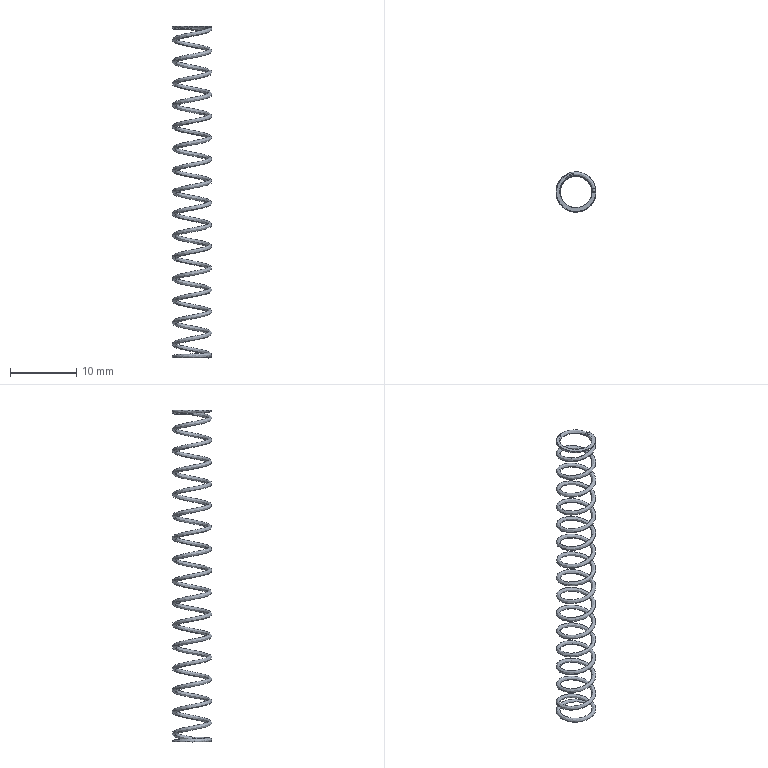Part | STEP file | 200 mesh_id542_x | 1 solid | 9 faces | box 5.998 x 5.997 x 50.45 mm | volume 76.992 mm3 | spline 5 | plane 4